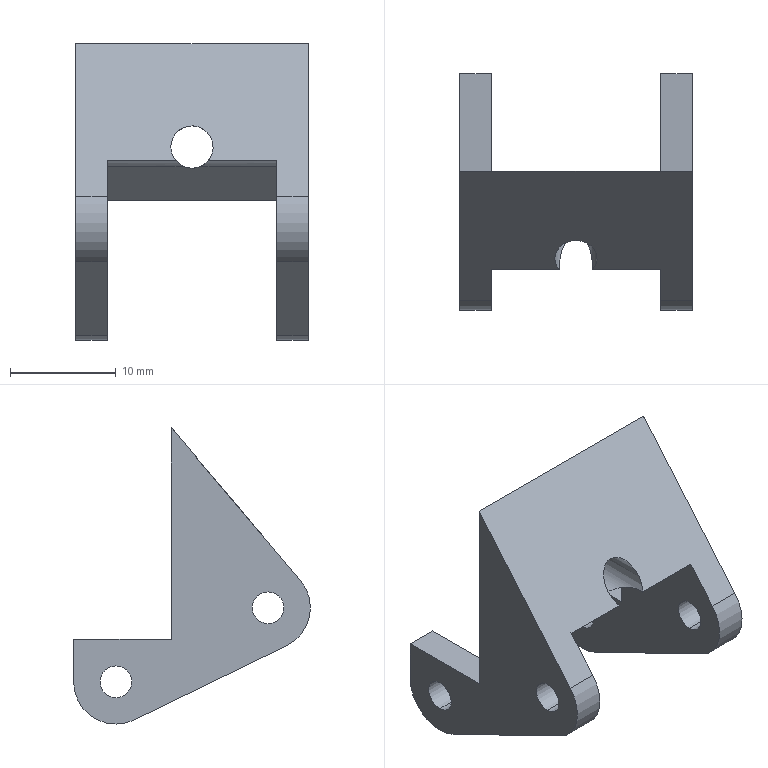Part | STEP file | DeraillieurCage End | 1 solid | 29 faces | box 22 x 22.387 x 28 mm | volume 2435 mm3 | cylinder 16 | plane 13 | commonest cylinder face diameters 3 x8 8 x4 4 x2 12 x2